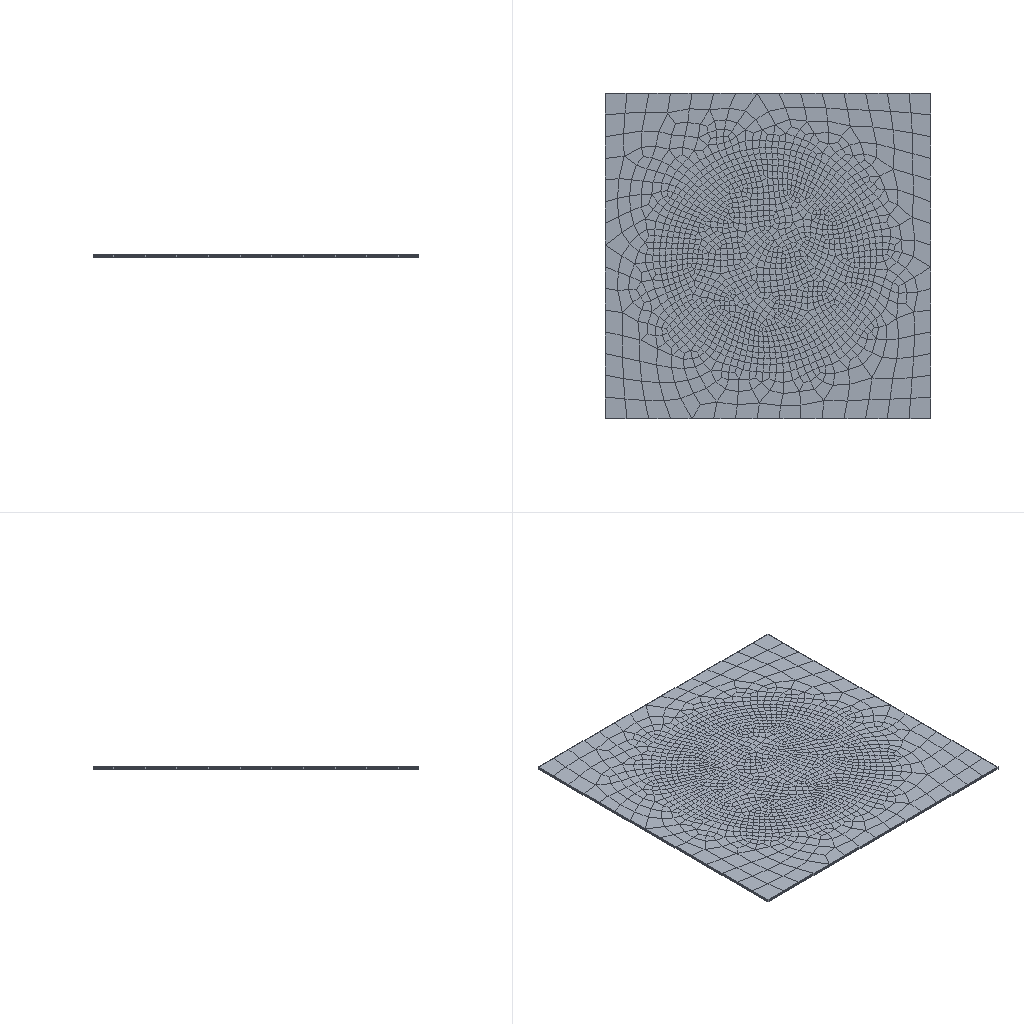Simulation study | abaqus
Set-up summary:
category,name,step,type,value,unit,region
solver,abaqus
solver,version,,,Abaqus/Explicit 2020
units,not stated in the deck,,not stated
analysis,deck,,transient,transient
load_step,Step-1,Step-1,transient
load_step,requested,,,1
mesh,nodes,,,11093
mesh,elements,,,9145
element_type,C3D8,,solid,8810
element_type,R3D3,,rigid,6
element_type,R3D4,,rigid,329
load,load commands in deck,,count,3
bc,support commands in deck,,count,12
material,MATERIAL-1,,in results
check,setup vs results,,match,"per instance, exact: element labels, types and connectivity; labels of the nodes the elements use; coordinates of those nodes at SINGLE_PRECISION in 2 of 2 instance(s)"
Abaqus input file, long lists of numbers shortened:
*Heading
** Job name: Job-1 Model name: Model-1
** Generated by: Abaqus/CAE 2020
*Preprint, echo=NO, model=NO, history=NO, contact=NO
**
** PARTS
**
*Part, name=ban
*Node
      1,           0.,           0.,           0.
      2,         150.,           0.,           0.
** (10756 more lines like these left out)
*Element, type=C3D8
   1,  662,  606,  556,  558, 4564, 4508, 4458, 4460
   2,  356,  504,  503,  429, 4258, 4406, 4405, 4331
** (8808 more lines like these left out)
*Nset, nset=Set-6, generate
     1,  10758,      1
*Elset, elset=Set-6, generate
    1,  8810,     1
** Section: Section-1
*Solid Section, elset=Set-6, material=Material-1
,
*End Part
**
*Part, name=rigid
*Node
      1,          -4.,           0.,           0.
      2,          -4.,           0.,           8.
** (332 more lines like these left out)
*Element, type=R3D4
  1,   1,  24,  47,  69
  2,  24,  23,  48,  47
** (327 more lines like these left out)
*Element, type=R3D3
162, 281, 200, 202
163, 276, 213, 275
** (4 more lines like these left out)
*Node
    335,           0., 2.44929371e-16,           8.
*Nset, nset=rigid-RefPt_, internal
335,
*Elset, elset=rigid, generate
   1,  335,    1
*End Part
**
**
** ASSEMBLY
**
*Assembly, name=Assembly
**
*Instance, name=ban-1, part=ban
*End Instance
**
*Instance, name=rigid-1, part=rigid
        115.,         -75.,          5.2
*End Instance
**
*Node
      1,          75.,         -75.,   1.2
*Node
      2,          75.,         -75.,   13.2
*Nset, nset=Set-1, instance=ban-1
    1,    2,    3,    4,    5,    6,    7,    8,    9,   10,   11,   12,   13,   14,   15,   16
   17,   18,   19,   20,   21,   22,   23,   24,   25,   26,   27,   28,   29,   30,   31,   32
** (228 more lines like these left out)
*Elset, elset=Set-1, instance=ban-1, generate
    1,  2650,     1
*Nset, nset=Set-4
 2,
*Nset, nset=Set-5, instance=rigid-1
 335,
*Nset, nset=Set-6, instance=ban-1
    1,    2,    3,    4,    5,    6,    7,    8,    9,   10,   11,   12,   13,   14,   15,   16
   17,   18,   19,   20,   21,   22,   23,   24,   25,   26,   27,   28,   29,   30,   31,   32
** (75 more lines like these left out)
*Elset, elset=Set-6, instance=ban-1
    1,    2,    3,    4,    5,    6,    7,    8,    9,   10,   11,   12,   13,   14,   15,   16
   17,   18,   19,   20,   21,   22,   23,   24,   25,   26,   27,   28,   29,   30,   31,   32
** (65 more lines like these left out)
*Nset, nset=Set-8
 1,
*Nset, nset=b_Set-2, instance=rigid-1, generate
   1,  334,    1
*Elset, elset=b_Set-2, instance=rigid-1, generate
   1,  335,    1
*Nset, nset=m_Set-7
 1,
*Nset, nset=_PickedSet13, internal
 2,
*Elset, elset=_m_Surf-1_SPOS, internal, instance=rigid-1, generate
   1,  272,    1
*Surface, type=ELEMENT, name=m_Surf-1
_m_Surf-1_SPOS, SPOS
*Elset, elset=_s_Surf-1_S1, internal, instance=ban-1, generate
 7579,  8810,     1
*Surface, type=ELEMENT, name=s_Surf-1
_s_Surf-1_S1, S1
*Elset, elset=_s_Surf-3_S2, internal, instance=ban-1, generate
 2121,  2650,     1
*Elset, elset=_s_Surf-3_S1, internal, instance=ban-1, generate
   1,  530,    1
*Surface, type=ELEMENT, name=s_Surf-3
_s_Surf-3_S2, S2
_s_Surf-3_S1, S1
*Rigid Body, ref node=rigid-1.rigid-RefPt_, elset=rigid-1.rigid
** Constraint: Constraint-2
*Coupling, constraint name=Constraint-2, ref node=m_Set-7, surface=s_Surf-3
*Kinematic
*End Assembly
**
** MATERIALS
**
*Material, name=Material-1
*Density
 2.2e-09,
*Elastic
5594., 0.324
*Plastic
116.,0.
**
** INTERACTION PROPERTIES
**
*Surface Interaction, name=IntProp-1
*Friction
 0.1,
*Surface Behavior, pressure-overclosure=HARD
** ----------------------------------------------------------------
**
** STEP: Step-1
**
*Step, name=Step-1, nlgeom=YES
*Dynamic, Explicit
, 10.
*Bulk Viscosity
0.06, 1.2
** Mass Scaling: Semi-Automatic
**               Whole Model
*Fixed Mass Scaling, factor=5000.
**
** BOUNDARY CONDITIONS
**
** Name: BC-2 Type: 速度/角速度
*Boundary, type=VELOCITY
Set-5, 1, 1, -3.
Set-5, 2, 2
Set-5, 3, 3, -4.
Set-5, 4, 4
Set-5, 5, 5
Set-5, 6, 6
** Name: BC-4 Type: 速度/角速度
*Boundary, type=VELOCITY
Set-8, 1, 1
Set-8, 2, 2
Set-8, 3, 3
Set-8, 4, 4
Set-8, 5, 5
Set-8, 6, 6, 62.8
**
** INTERACTIONS
**
** Interaction: Int-1
*Contact Pair, interaction=IntProp-1, mechanical constraint=KINEMATIC, cpset=Int-1
m_Surf-1, s_Surf-1
**
** OUTPUT REQUESTS
**
*Restart, write, number interval=1, time marks=NO
**
** FIELD OUTPUT: F-Output-1
**
*Output, field, number interval=200
*Node Output
A, CF, RF, U, V
*Element Output, directions=YES
E, LE, MISES, PE, PEEQ, PEMAG, S
*Contact Output
CDISP, CSTRESS
**
** HISTORY OUTPUT: H-Output-1
**
*Output, history, variable=PRESELECT
*End Step
Results summary:
result,step,Step-1,completed,increments=2892861 time=10.0/10.0
result,analysis,,,transient
result,last_loadstep,,,1
result,primary field,,,U
result,reaction total,,FX,-624.723,model units
result,reaction total,,FY,1044.483,model units
result,reaction total,,FZ,294.661,model units